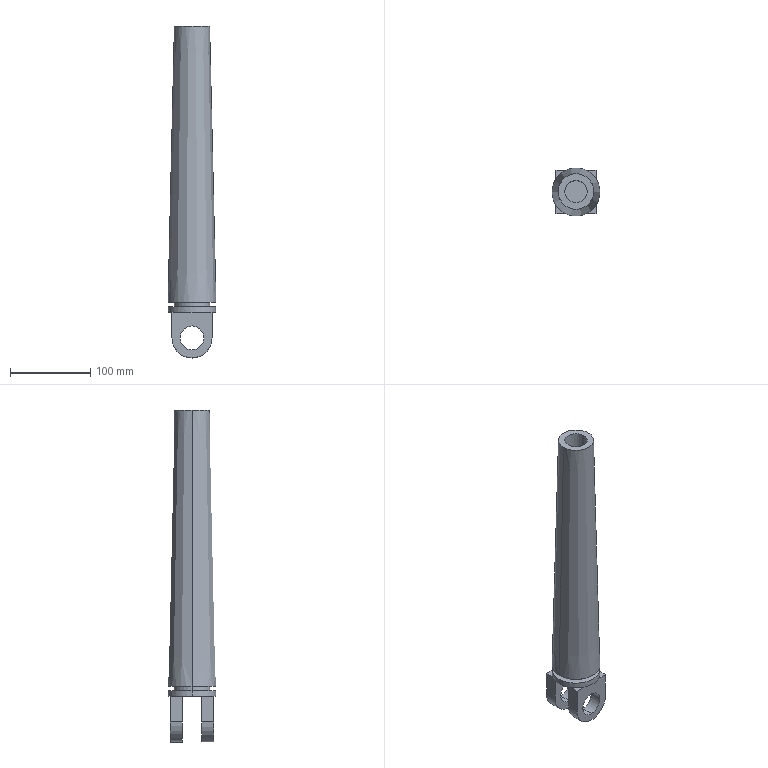Part | SolidWorks | features Extrusion 1, MirrorPattern 1, Revolution 1 | 1 solid | 34 faces | box 59.866 x 59.866 x 414.086 mm | volume 604728 mm3 | plane 19 | cylinder 13 | cone 2 | commonest cylinder face diameters 30 x4 50 x3 28 x2 44.765 x2 59.866 x2
STEP:
#1=CARTESIAN_POINT('',(0.,-39.,-15.));
#2=VERTEX_POINT('',#1);
#3=CARTESIAN_POINT('',(0.,-39.,15.));
#4=VERTEX_POINT('',#3);
#5=CARTESIAN_POINT('',(0.,-39.,0.));
#6=DIRECTION('',(0.,1.,0.));
#7=DIRECTION('',(0.,0.,1.));
#8=AXIS2_PLACEMENT_3D('',#5,#6,#7);
#9=CIRCLE('',#8,15.);
#10=EDGE_CURVE('',#2,#4,#9,.T.);
#11=ORIENTED_EDGE('',*,*,#10,.F.);
#12=CARTESIAN_POINT('',(0.,-24.,-15.));
#13=VERTEX_POINT('',#12);
#14=CARTESIAN_POINT('',(0.,-39.,-15.));
#15=DIRECTION('',(0.,1.,0.));
#16=VECTOR('',#15,1000.);
#17=LINE('',#14,#16);
#18=EDGE_CURVE('',#2,#13,#17,.T.);
#19=ORIENTED_EDGE('',*,*,#18,.T.);
#20=CARTESIAN_POINT('',(0.,-24.,15.));
#21=VERTEX_POINT('',#20);
#22=CARTESIAN_POINT('',(0.,-24.,0.));
#23=DIRECTION('',(0.,1.,0.));
#24=DIRECTION('',(0.,0.,1.));
#25=AXIS2_PLACEMENT_3D('',#22,#23,#24);
#26=CIRCLE('',#25,15.);
#27=EDGE_CURVE('',#13,#21,#26,.T.);
#28=ORIENTED_EDGE('',*,*,#27,.T.);
#29=CARTESIAN_POINT('',(0.,-39.,15.));
#30=DIRECTION('',(0.,1.,0.));
#31=VECTOR('',#30,1000.);
#32=LINE('',#29,#31);
#33=EDGE_CURVE('',#4,#21,#32,.T.);
#34=ORIENTED_EDGE('',*,*,#33,.F.);
#35=EDGE_LOOP('',(#11,#19,#28,#34));
#36=FACE_OUTER_BOUND('',#35,.T.);
#37=CARTESIAN_POINT('',(0.,-39.,0.));
#38=DIRECTION('',(0.,1.,0.));
#39=DIRECTION('',(0.,0.,1.));
#40=AXIS2_PLACEMENT_3D('',#37,#38,#39);
#41=CYLINDRICAL_SURFACE('',#40,15.);
#42=ADVANCED_FACE('',(#36),#41,.F.);
#43=CARTESIAN_POINT('',(-29.933,-12.,39.086));
#44=VERTEX_POINT('',#43);
#45=CARTESIAN_POINT('',(29.933,-12.,39.086));
#46=VERTEX_POINT('',#45);
#47=CARTESIAN_POINT('',(0.,-12.,39.086));
#48=DIRECTION('',(0.,0.,-1.));
#49=DIRECTION('',(-1.,0.,0.));
#50=AXIS2_PLACEMENT_3D('',#47,#48,#49);
#51=CIRCLE('',#50,29.933);
#52=EDGE_CURVE('',#44,#46,#51,.T.);
#53=ORIENTED_EDGE('',*,*,#52,.T.);
#54=CARTESIAN_POINT('',(29.933,-12.,31.913));
#55=VERTEX_POINT('',#54);
#56=CARTESIAN_POINT('',(29.933,-12.,31.913));
#57=DIRECTION('',(0.,0.,-1.));
#58=VECTOR('',#57,1000.);
#59=LINE('',#56,#58);
#60=EDGE_CURVE('',#46,#55,#59,.T.);
#61=ORIENTED_EDGE('',*,*,#60,.T.);
#62=CARTESIAN_POINT('',(25.,4.462,31.913));
#63=VERTEX_POINT('',#62);
#64=CARTESIAN_POINT('',(0.,-12.,31.913));
#65=DIRECTION('',(0.,0.,-1.));
#66=DIRECTION('',(-1.,0.,0.));
#67=AXIS2_PLACEMENT_3D('',#64,#65,#66);
#68=CIRCLE('',#67,29.933);
#69=EDGE_CURVE('',#63,#55,#68,.T.);
#70=ORIENTED_EDGE('',*,*,#69,.F.);
#71=CARTESIAN_POINT('',(12.923,15.,31.913));
#72=VERTEX_POINT('',#71);
#73=CARTESIAN_POINT('',(0.,-12.,31.913));
#74=DIRECTION('',(0.,0.,-1.));
#75=DIRECTION('',(-1.,0.,0.));
#76=AXIS2_PLACEMENT_3D('',#73,#74,#75);
#77=CIRCLE('',#76,29.933);
#78=EDGE_CURVE('',#72,#63,#77,.T.);
#79=ORIENTED_EDGE('',*,*,#78,.F.);
#80=CARTESIAN_POINT('',(-12.923,15.,31.913));
#81=VERTEX_POINT('',#80);
#82=CARTESIAN_POINT('',(0.,-12.,31.913));
#83=DIRECTION('',(0.,0.,-1.));
#84=DIRECTION('',(-1.,0.,0.));
#85=AXIS2_PLACEMENT_3D('',#82,#83,#84);
#86=CIRCLE('',#85,29.933);
#87=EDGE_CURVE('',#81,#72,#86,.T.);
#88=ORIENTED_EDGE('',*,*,#87,.F.);
#89=CARTESIAN_POINT('',(-25.,4.462,31.913));
#90=VERTEX_POINT('',#89);
#91=CARTESIAN_POINT('',(0.,-12.,31.913));
#92=DIRECTION('',(0.,0.,-1.));
#93=DIRECTION('',(-1.,0.,0.));
#94=AXIS2_PLACEMENT_3D('',#91,#92,#93);
#95=CIRCLE('',#94,29.933);
#96=EDGE_CURVE('',#90,#81,#95,.T.);
#97=ORIENTED_EDGE('',*,*,#96,.F.);
#98=CARTESIAN_POINT('',(-29.933,-12.,31.913));
#99=VERTEX_POINT('',#98);
#100=CARTESIAN_POINT('',(0.,-12.,31.913));
#101=DIRECTION('',(0.,0.,-1.));
#102=DIRECTION('',(-1.,0.,0.));
#103=AXIS2_PLACEMENT_3D('',#100,#101,#102);
#104=CIRCLE('',#103,29.933);
#105=EDGE_CURVE('',#99,#90,#104,.T.);
#106=ORIENTED_EDGE('',*,*,#105,.F.);
#107=CARTESIAN_POINT('',(-29.933,-12.,31.913));
#108=DIRECTION('',(0.,0.,-1.));
#109=VECTOR('',#108,1000.);
#110=LINE('',#107,#109);
#111=EDGE_CURVE('',#44,#99,#110,.T.);
#112=ORIENTED_EDGE('',*,*,#111,.F.);
#113=EDGE_LOOP('',(#53,#61,#70,#79,#88,#97,#106,#112));
#114=FACE_OUTER_BOUND('',#113,.T.);
#115=CARTESIAN_POINT('',(0.,-12.,31.913));
#116=DIRECTION('',(0.,0.,-1.));
#117=DIRECTION('',(-1.,0.,0.));
#118=AXIS2_PLACEMENT_3D('',#115,#116,#117);
#119=CYLINDRICAL_SURFACE('',#118,29.933);
#120=ADVANCED_FACE('',(#114),#119,.T.);
#121=CARTESIAN_POINT('',(-22.383,-12.,44.842));
#122=VERTEX_POINT('',#121);
#123=CARTESIAN_POINT('',(22.383,-12.,44.842));
#124=VERTEX_POINT('',#123);
#125=CARTESIAN_POINT('',(0.,-12.,44.842));
#126=DIRECTION('',(0.,0.,-1.));
#127=DIRECTION('',(-1.,0.,0.));
#128=AXIS2_PLACEMENT_3D('',#125,#126,#127);
#129=CIRCLE('',#128,22.383);
#130=EDGE_CURVE('',#122,#124,#129,.T.);
#131=ORIENTED_EDGE('',*,*,#130,.T.);
#132=CARTESIAN_POINT('',(22.383,-12.,39.086));
#133=VERTEX_POINT('',#132);
#134=CARTESIAN_POINT('',(22.383,-12.,31.913));
#135=DIRECTION('',(0.,0.,-1.));
#136=VECTOR('',#135,1000.);
#137=LINE('',#134,#136);
#138=EDGE_CURVE('',#124,#133,#137,.T.);
#139=ORIENTED_EDGE('',*,*,#138,.T.);
#140=CARTESIAN_POINT('',(-22.383,-12.,39.086));
#141=VERTEX_POINT('',#140);
#142=CARTESIAN_POINT('',(0.,-12.,39.086));
#143=DIRECTION('',(0.,0.,-1.));
#144=DIRECTION('',(-1.,0.,0.));
#145=AXIS2_PLACEMENT_3D('',#142,#143,#144);
#146=CIRCLE('',#145,22.383);
#147=EDGE_CURVE('',#141,#133,#146,.T.);
#148=ORIENTED_EDGE('',*,*,#147,.F.);
#149=CARTESIAN_POINT('',(-22.383,-12.,31.913));
#150=DIRECTION('',(0.,0.,-1.));
#151=VECTOR('',#150,1000.);
#152=LINE('',#149,#151);
#153=EDGE_CURVE('',#122,#141,#152,.T.);
#154=ORIENTED_EDGE('',*,*,#153,.F.);
#155=EDGE_LOOP('',(#131,#139,#148,#154));
#156=FACE_OUTER_BOUND('',#155,.T.);
#157=CARTESIAN_POINT('',(0.,-12.,31.913));
#158=DIRECTION('',(0.,0.,-1.));
#159=DIRECTION('',(-1.,0.,0.));
#160=AXIS2_PLACEMENT_3D('',#157,#158,#159);
#161=CYLINDRICAL_SURFACE('',#160,22.383);
#162=ADVANCED_FACE('',(#156),#161,.T.);
#163=CARTESIAN_POINT('',(-22.,-12.,389.086));
#164=VERTEX_POINT('',#163);
#165=CARTESIAN_POINT('',(22.,-12.,389.086));
#166=VERTEX_POINT('',#165);
#167=CARTESIAN_POINT('',(0.,-12.,389.086));
#168=DIRECTION('',(0.,0.,-1.));
#169=DIRECTION('',(-1.,0.,0.));
#170=AXIS2_PLACEMENT_3D('',#167,#168,#169);
#171=CIRCLE('',#170,22.);
#172=EDGE_CURVE('',#164,#166,#171,.T.);
#173=ORIENTED_EDGE('',*,*,#172,.T.);
#174=CARTESIAN_POINT('',(29.933,-12.,44.842));
#175=VERTEX_POINT('',#174);
#176=CARTESIAN_POINT('',(22.,-12.,389.086));
#177=DIRECTION('',(0.02304,0.,-0.9997));
#178=VECTOR('',#177,1000.);
#179=LINE('',#176,#178);
#180=EDGE_CURVE('',#166,#175,#179,.T.);
#181=ORIENTED_EDGE('',*,*,#180,.T.);
#182=CARTESIAN_POINT('',(-29.933,-12.,44.842));
#183=VERTEX_POINT('',#182);
#184=CARTESIAN_POINT('',(0.,-12.,44.842));
#185=DIRECTION('',(0.,0.,-1.));
#186=DIRECTION('',(-1.,0.,0.));
#187=AXIS2_PLACEMENT_3D('',#184,#185,#186);
#188=CIRCLE('',#187,29.933);
#189=EDGE_CURVE('',#183,#175,#188,.T.);
#190=ORIENTED_EDGE('',*,*,#189,.F.);
#191=CARTESIAN_POINT('',(-22.,-12.,389.086));
#192=DIRECTION('',(-0.02304,0.,-0.9997));
#193=VECTOR('',#192,1000.);
#194=LINE('',#191,#193);
#195=EDGE_CURVE('',#164,#183,#194,.T.);
#196=ORIENTED_EDGE('',*,*,#195,.F.);
#197=EDGE_LOOP('',(#173,#181,#190,#196));
#198=FACE_OUTER_BOUND('',#197,.T.);
#199=CARTESIAN_POINT('',(0.,-12.,389.086));
#200=DIRECTION('',(0.,0.,-1.));
#201=DIRECTION('',(-1.,0.,0.));
#202=AXIS2_PLACEMENT_3D('',#199,#200,#201);
#203=CONICAL_SURFACE('',#202,22.,0.02304);
#204=ADVANCED_FACE('',(#198),#203,.T.);
#205=CARTESIAN_POINT('',(14.,-12.,389.086));
#206=VERTEX_POINT('',#205);
#207=CARTESIAN_POINT('',(-14.,-12.,389.086));
#208=VERTEX_POINT('',#207);
#209=CARTESIAN_POINT('',(0.,-12.,389.086));
#210=DIRECTION('',(0.,0.,-1.));
#211=DIRECTION('',(-1.,0.,0.));
#212=AXIS2_PLACEMENT_3D('',#209,#210,#211);
#213=CIRCLE('',#212,14.);
#214=EDGE_CURVE('',#206,#208,#213,.T.);
#215=ORIENTED_EDGE('',*,*,#214,.F.);
#216=CARTESIAN_POINT('',(14.,-12.,39.086));
#217=VERTEX_POINT('',#216);
#218=CARTESIAN_POINT('',(14.,-12.,31.913));
#219=DIRECTION('',(0.,0.,-1.));
#220=VECTOR('',#219,1000.);
#221=LINE('',#218,#220);
#222=EDGE_CURVE('',#206,#217,#221,.T.);
#223=ORIENTED_EDGE('',*,*,#222,.T.);
#224=CARTESIAN_POINT('',(-14.,-12.,39.086));
#225=VERTEX_POINT('',#224);
#226=CARTESIAN_POINT('',(0.,-12.,39.086));
#227=DIRECTION('',(0.,0.,-1.));
#228=DIRECTION('',(-1.,0.,0.));
#229=AXIS2_PLACEMENT_3D('',#226,#227,#228);
#230=CIRCLE('',#229,14.);
#231=EDGE_CURVE('',#217,#225,#230,.T.);
#232=ORIENTED_EDGE('',*,*,#231,.T.);
#233=CARTESIAN_POINT('',(-14.,-12.,31.913));
#234=DIRECTION('',(0.,0.,-1.));
#235=VECTOR('',#234,1000.);
#236=LINE('',#233,#235);
#237=EDGE_CURVE('',#208,#225,#236,.T.);
#238=ORIENTED_EDGE('',*,*,#237,.F.);
#239=EDGE_LOOP('',(#215,#223,#232,#238));
#240=FACE_OUTER_BOUND('',#239,.T.);
#241=CARTESIAN_POINT('',(0.,-12.,31.913));
#242=DIRECTION('',(0.,0.,-1.));
#243=DIRECTION('',(-1.,0.,0.));
#244=AXIS2_PLACEMENT_3D('',#241,#242,#243);
#245=CYLINDRICAL_SURFACE('',#244,14.);
#246=ADVANCED_FACE('',(#240),#245,.F.);
#247=CARTESIAN_POINT('',(0.,15.,-15.));
#248=VERTEX_POINT('',#247);
#249=CARTESIAN_POINT('',(0.,15.,15.));
#250=VERTEX_POINT('',#249);
#251=CARTESIAN_POINT('',(0.,15.,0.));
#252=DIRECTION('',(0.,1.,0.));
#253=DIRECTION('',(0.,0.,1.));
#254=AXIS2_PLACEMENT_3D('',#251,#252,#253);
#255=CIRCLE('',#254,15.);
#256=EDGE_CURVE('',#248,#250,#255,.T.);
#257=ORIENTED_EDGE('',*,*,#256,.T.);
#258=CARTESIAN_POINT('',(0.,0.,15.));
#259=VERTEX_POINT('',#258);
#260=CARTESIAN_POINT('',(0.,15.,15.));
#261=DIRECTION('',(0.,-1.,0.));
#262=VECTOR('',#261,1000.);
#263=LINE('',#260,#262);
#264=EDGE_CURVE('',#250,#259,#263,.T.);
#265=ORIENTED_EDGE('',*,*,#264,.T.);
#266=CARTESIAN_POINT('',(0.,0.,-15.));
#267=VERTEX_POINT('',#266);
#268=CARTESIAN_POINT('',(0.,0.,0.));
#269=DIRECTION('',(0.,1.,0.));
#270=DIRECTION('',(0.,0.,1.));
#271=AXIS2_PLACEMENT_3D('',#268,#269,#270);
#272=CIRCLE('',#271,15.);
#273=EDGE_CURVE('',#267,#259,#272,.T.);
#274=ORIENTED_EDGE('',*,*,#273,.F.);
#275=CARTESIAN_POINT('',(0.,15.,-15.));
#276=DIRECTION('',(0.,-1.,0.));
#277=VECTOR('',#276,1000.);
#278=LINE('',#275,#277);
#279=EDGE_CURVE('',#248,#267,#278,.T.);
#280=ORIENTED_EDGE('',*,*,#279,.F.);
#281=EDGE_LOOP('',(#257,#265,#274,#280));
#282=FACE_OUTER_BOUND('',#281,.T.);
#283=CARTESIAN_POINT('',(0.,15.,0.));
#284=DIRECTION('',(0.,-1.,0.));
#285=DIRECTION('',(0.,0.,-1.));
#286=AXIS2_PLACEMENT_3D('',#283,#284,#285);
#287=CYLINDRICAL_SURFACE('',#286,15.);
#288=ADVANCED_FACE('',(#282),#287,.F.);
#289=CARTESIAN_POINT('',(0.,15.,-25.));
#290=VERTEX_POINT('',#289);
#291=CARTESIAN_POINT('',(-25.,15.,0.));
#292=VERTEX_POINT('',#291);
#293=CARTESIAN_POINT('',(0.,15.,0.));
#294=DIRECTION('',(0.,1.,0.));
#295=DIRECTION('',(0.,0.,1.));
#296=AXIS2_PLACEMENT_3D('',#293,#294,#295);
#297=CIRCLE('',#296,25.);
#298=EDGE_CURVE('',#290,#292,#297,.T.);
#299=ORIENTED_EDGE('',*,*,#298,.F.);
#300=CARTESIAN_POINT('',(0.,0.,-25.));
#301=VERTEX_POINT('',#300);
#302=CARTESIAN_POINT('',(0.,15.,-25.));
#303=DIRECTION('',(0.,-1.,0.));
#304=VECTOR('',#303,1000.);
#305=LINE('',#302,#304);
#306=EDGE_CURVE('',#290,#301,#305,.T.);
#307=ORIENTED_EDGE('',*,*,#306,.T.);
#308=CARTESIAN_POINT('',(-25.,0.,0.));
#309=VERTEX_POINT('',#308);
#310=CARTESIAN_POINT('',(0.,0.,0.));
#311=DIRECTION('',(0.,1.,0.));
#312=DIRECTION('',(0.,0.,1.));
#313=AXIS2_PLACEMENT_3D('',#310,#311,#312);
#314=CIRCLE('',#313,25.);
#315=EDGE_CURVE('',#301,#309,#314,.T.);
#316=ORIENTED_EDGE('',*,*,#315,.T.);
#317=CARTESIAN_POINT('',(-25.,15.,0.));
#318=DIRECTION('',(0.,-1.,0.));
#319=VECTOR('',#318,1000.);
#320=LINE('',#317,#319);
#321=EDGE_CURVE('',#292,#309,#320,.T.);
#322=ORIENTED_EDGE('',*,*,#321,.F.);
#323=EDGE_LOOP('',(#299,#307,#316,#322));
#324=FACE_OUTER_BOUND('',#323,.T.);
#325=CARTESIAN_POINT('',(0.,15.,0.));
#326=DIRECTION('',(0.,-1.,0.));
#327=DIRECTION('',(0.,0.,-1.));
#328=AXIS2_PLACEMENT_3D('',#325,#326,#327);
#329=CYLINDRICAL_SURFACE('',#328,25.);
#330=ADVANCED_FACE('',(#324),#329,.T.);
#331=CARTESIAN_POINT('',(12.923,-39.,31.913));
#332=VERTEX_POINT('',#331);
#333=CARTESIAN_POINT('',(-12.923,-39.,31.913));
#334=VERTEX_POINT('',#333);
#335=CARTESIAN_POINT('',(0.,-12.,31.913));
#336=DIRECTION('',(0.,0.,-1.));
#337=DIRECTION('',(-1.,0.,0.));
#338=AXIS2_PLACEMENT_3D('',#335,#336,#337);
#339=CIRCLE('',#338,29.933);
#340=EDGE_CURVE('',#332,#334,#339,.T.);
#341=ORIENTED_EDGE('',*,*,#340,.T.);
#342=CARTESIAN_POINT('',(0.,-39.,31.913));
#343=DIRECTION('',(1.,0.,0.));
#344=VECTOR('',#343,1000.);
#345=LINE('',#342,#344);
#346=EDGE_CURVE('',#334,#332,#345,.T.);
#347=ORIENTED_EDGE('',*,*,#346,.T.);
#348=EDGE_LOOP('',(#341,#347));
#349=FACE_OUTER_BOUND('',#348,.T.);
#350=CARTESIAN_POINT('',(0.,-12.,31.913));
#351=DIRECTION('',(0.,0.,1.));
#352=DIRECTION('',(1.,0.,0.));
#353=AXIS2_PLACEMENT_3D('',#350,#351,#352);
#354=PLANE('',#353);
#355=ADVANCED_FACE('',(#349),#354,.F.);
#356=CARTESIAN_POINT('',(-25.,15.,31.913));
#357=VERTEX_POINT('',#356);
#358=CARTESIAN_POINT('',(-25.,15.,31.913));
#359=DIRECTION('',(0.,-1.,0.));
#360=VECTOR('',#359,1000.);
#361=LINE('',#358,#360);
#362=EDGE_CURVE('',#357,#90,#361,.T.);
#363=ORIENTED_EDGE('',*,*,#362,.T.);
#364=ORIENTED_EDGE('',*,*,#96,.T.);
#365=CARTESIAN_POINT('',(-25.,15.,31.913));
#366=DIRECTION('',(1.,0.,0.));
#367=VECTOR('',#366,1000.);
#368=LINE('',#365,#367);
#369=EDGE_CURVE('',#357,#81,#368,.T.);
#370=ORIENTED_EDGE('',*,*,#369,.F.);
#371=EDGE_LOOP('',(#363,#364,#370));
#372=FACE_OUTER_BOUND('',#371,.T.);
#373=CARTESIAN_POINT('',(-25.,15.,31.913));
#374=DIRECTION('',(0.,0.,-1.));
#375=DIRECTION('',(-1.,0.,0.));
#376=AXIS2_PLACEMENT_3D('',#373,#374,#375);
#377=PLANE('',#376);
#378=ADVANCED_FACE('',(#372),#377,.F.);
#379=CARTESIAN_POINT('',(25.,15.,0.));
#380=VERTEX_POINT('',#379);
#381=CARTESIAN_POINT('',(0.,15.,0.));
#382=DIRECTION('',(0.,1.,0.));
#383=DIRECTION('',(0.,0.,1.));
#384=AXIS2_PLACEMENT_3D('',#381,#382,#383);
#385=CIRCLE('',#384,25.);
#386=EDGE_CURVE('',#380,#290,#385,.T.);
#387=ORIENTED_EDGE('',*,*,#386,.T.);
#388=ORIENTED_EDGE('',*,*,#298,.T.);
#389=CARTESIAN_POINT('',(-25.,15.,0.));
#390=DIRECTION('',(0.,0.,1.));
#391=VECTOR('',#390,1000.);
#392=LINE('',#389,#391);
#393=EDGE_CURVE('',#292,#357,#392,.T.);
#394=ORIENTED_EDGE('',*,*,#393,.T.);
#395=ORIENTED_EDGE('',*,*,#369,.T.);
#396=CARTESIAN_POINT('',(-25.,15.,31.913));
#397=DIRECTION('',(1.,0.,0.));
#398=VECTOR('',#397,1000.);
#399=LINE('',#396,#398);
#400=EDGE_CURVE('',#81,#72,#399,.T.);
#401=ORIENTED_EDGE('',*,*,#400,.T.);
#402=CARTESIAN_POINT('',(25.,15.,31.913));
#403=VERTEX_POINT('',#402);
#404=CARTESIAN_POINT('',(-25.,15.,31.913));
#405=DIRECTION('',(1.,0.,0.));
#406=VECTOR('',#405,1000.);
#407=LINE('',#404,#406);
#408=EDGE_CURVE('',#72,#403,#407,.T.);
#409=ORIENTED_EDGE('',*,*,#408,.T.);
#410=CARTESIAN_POINT('',(25.,15.,0.));
#411=DIRECTION('',(0.,0.,-1.));
#412=VECTOR('',#411,1000.);
#413=LINE('',#410,#412);
#414=EDGE_CURVE('',#403,#380,#413,.T.);
#415=ORIENTED_EDGE('',*,*,#414,.T.);
#416=EDGE_LOOP('',(#387,#388,#394,#395,#401,#409,#415));
#417=FACE_OUTER_BOUND('',#416,.T.);
#418=ORIENTED_EDGE('',*,*,#256,.F.);
#419=CARTESIAN_POINT('',(0.,15.,0.));
#420=DIRECTION('',(0.,1.,0.));
#421=DIRECTION('',(0.,0.,1.));
#422=AXIS2_PLACEMENT_3D('',#419,#420,#421);
#423=CIRCLE('',#422,15.);
#424=EDGE_CURVE('',#250,#248,#423,.T.);
#425=ORIENTED_EDGE('',*,*,#424,.F.);
#426=EDGE_LOOP('',(#418,#425));
#427=FACE_BOUND('',#426,.T.);
#428=CARTESIAN_POINT('',(0.,15.,0.));
#429=DIRECTION('',(0.,1.,0.));
#430=DIRECTION('',(0.,0.,1.));
#431=AXIS2_PLACEMENT_3D('',#428,#429,#430);
#432=PLANE('',#431);
#433=ADVANCED_FACE('',(#417,#427),#432,.T.);
#434=CARTESIAN_POINT('',(25.,0.,0.));
#435=VERTEX_POINT('',#434);
#436=CARTESIAN_POINT('',(0.,0.,0.));
#437=DIRECTION('',(0.,1.,0.));
#438=DIRECTION('',(0.,0.,1.));
#439=AXIS2_PLACEMENT_3D('',#436,#437,#438);
#440=CIRCLE('',#439,25.);
#441=EDGE_CURVE('',#435,#301,#440,.T.);
#442=ORIENTED_EDGE('',*,*,#441,.F.);
#443=CARTESIAN_POINT('',(25.,0.,31.913));
#444=VERTEX_POINT('',#443);
#445=CARTESIAN_POINT('',(25.,0.,0.));
#446=DIRECTION('',(0.,0.,-1.));
#447=VECTOR('',#446,1000.);
#448=LINE('',#445,#447);
#449=EDGE_CURVE('',#444,#435,#448,.T.);
#450=ORIENTED_EDGE('',*,*,#449,.F.);
#451=CARTESIAN_POINT('',(-25.,0.,31.913));
#452=VERTEX_POINT('',#451);
#453=CARTESIAN_POINT('',(-25.,0.,31.913));
#454=DIRECTION('',(1.,0.,0.));
#455=VECTOR('',#454,1000.);
#456=LINE('',#453,#455);
#457=EDGE_CURVE('',#452,#444,#456,.T.);
#458=ORIENTED_EDGE('',*,*,#457,.F.);
#459=CARTESIAN_POINT('',(-25.,0.,0.));
#460=DIRECTION('',(0.,0.,1.));
#461=VECTOR('',#460,1000.);
#462=LINE('',#459,#461);
#463=EDGE_CURVE('',#309,#452,#462,.T.);
#464=ORIENTED_EDGE('',*,*,#463,.F.);
#465=ORIENTED_EDGE('',*,*,#315,.F.);
#466=EDGE_LOOP('',(#442,#450,#458,#464,#465));
#467=FACE_OUTER_BOUND('',#466,.T.);
#468=ORIENTED_EDGE('',*,*,#273,.T.);
#469=CARTESIAN_POINT('',(0.,0.,0.));
#470=DIRECTION('',(0.,1.,0.));
#471=DIRECTION('',(0.,0.,1.));
#472=AXIS2_PLACEMENT_3D('',#469,#470,#471);
#473=CIRCLE('',#472,15.);
#474=EDGE_CURVE('',#259,#267,#473,.T.);
#475=ORIENTED_EDGE('',*,*,#474,.T.);
#476=EDGE_LOOP('',(#468,#475));
#477=FACE_BOUND('',#476,.T.);
#478=CARTESIAN_POINT('',(0.,0.,0.));
#479=DIRECTION('',(0.,1.,0.));
#480=DIRECTION('',(0.,0.,1.));
#481=AXIS2_PLACEMENT_3D('',#478,#479,#480);
#482=PLANE('',#481);
#483=ADVANCED_FACE('',(#467,#477),#482,.F.);
#484=ORIENTED_EDGE('',*,*,#306,.F.);
#485=ORIENTED_EDGE('',*,*,#386,.F.);
#486=CARTESIAN_POINT('',(25.,15.,0.));
#487=DIRECTION('',(0.,-1.,0.));
#488=VECTOR('',#487,1000.);
#489=LINE('',#486,#488);
#490=EDGE_CURVE('',#380,#435,#489,.T.);
#491=ORIENTED_EDGE('',*,*,#490,.T.);
#492=ORIENTED_EDGE('',*,*,#441,.T.);
#493=EDGE_LOOP('',(#484,#485,#491,#492));
#494=FACE_OUTER_BOUND('',#493,.T.);
#495=CARTESIAN_POINT('',(0.,15.,0.));
#496=DIRECTION('',(0.,-1.,0.));
#497=DIRECTION('',(0.,0.,-1.));
#498=AXIS2_PLACEMENT_3D('',#495,#496,#497);
#499=CYLINDRICAL_SURFACE('',#498,25.);
#500=ADVANCED_FACE('',(#494),#499,.T.);
#501=ORIENTED_EDGE('',*,*,#463,.T.);
#502=CARTESIAN_POINT('',(-25.,15.,31.913));
#503=DIRECTION('',(0.,-1.,0.));
#504=VECTOR('',#503,1000.);
#505=LINE('',#502,#504);
#506=EDGE_CURVE('',#90,#452,#505,.T.);
#507=ORIENTED_EDGE('',*,*,#506,.F.);
#508=ORIENTED_EDGE('',*,*,#362,.F.);
#509=ORIENTED_EDGE('',*,*,#393,.F.);
#510=ORIENTED_EDGE('',*,*,#321,.T.);
#511=EDGE_LOOP('',(#501,#507,#508,#509,#510));
#512=FACE_OUTER_BOUND('',#511,.T.);
#513=CARTESIAN_POINT('',(-25.,15.,0.));
#514=DIRECTION('',(1.,0.,0.));
#515=DIRECTION('',(0.,0.,-1.));
#516=AXIS2_PLACEMENT_3D('',#513,#514,#515);
#517=PLANE('',#516);
#518=ADVANCED_FACE('',(#512),#517,.F.);
#519=ORIENTED_EDGE('',*,*,#408,.F.);
#520=ORIENTED_EDGE('',*,*,#78,.T.);
#521=CARTESIAN_POINT('',(25.,15.,31.913));
#522=DIRECTION('',(0.,-1.,0.));
#523=VECTOR('',#522,1000.);
#524=LINE('',#521,#523);
#525=EDGE_CURVE('',#403,#63,#524,.T.);
#526=ORIENTED_EDGE('',*,*,#525,.F.);
#527=EDGE_LOOP('',(#519,#520,#526));
#528=FACE_OUTER_BOUND('',#527,.T.);
#529=CARTESIAN_POINT('',(-25.,15.,31.913));
#530=DIRECTION('',(0.,0.,-1.));
#531=DIRECTION('',(-1.,0.,0.));
#532=AXIS2_PLACEMENT_3D('',#529,#530,#531);
#533=PLANE('',#532);
#534=ADVANCED_FACE('',(#528),#533,.F.);
#535=ORIENTED_EDGE('',*,*,#449,.T.);
#536=ORIENTED_EDGE('',*,*,#490,.F.);
#537=ORIENTED_EDGE('',*,*,#414,.F.);
#538=ORIENTED_EDGE('',*,*,#525,.T.);
#539=CARTESIAN_POINT('',(25.,15.,31.913));
#540=DIRECTION('',(0.,-1.,0.));
#541=VECTOR('',#540,1000.);
#542=LINE('',#539,#541);
#543=EDGE_CURVE('',#63,#444,#542,.T.);
#544=ORIENTED_EDGE('',*,*,#543,.T.);
#545=EDGE_LOOP('',(#535,#536,#537,#538,#544));
#546=FACE_OUTER_BOUND('',#545,.T.);
#547=CARTESIAN_POINT('',(25.,15.,0.));
#548=DIRECTION('',(-1.,0.,0.));
#549=DIRECTION('',(0.,0.,1.));
#550=AXIS2_PLACEMENT_3D('',#547,#548,#549);
#551=PLANE('',#550);
#552=ADVANCED_FACE('',(#546),#551,.F.);
#553=ORIENTED_EDGE('',*,*,#264,.F.);
#554=ORIENTED_EDGE('',*,*,#424,.T.);
#555=ORIENTED_EDGE('',*,*,#279,.T.);
#556=ORIENTED_EDGE('',*,*,#474,.F.);
#557=EDGE_LOOP('',(#553,#554,#555,#556));
#558=FACE_OUTER_BOUND('',#557,.T.);
#559=CARTESIAN_POINT('',(0.,15.,0.));
#560=DIRECTION('',(0.,-1.,0.));
#561=DIRECTION('',(0.,0.,-1.));
#562=AXIS2_PLACEMENT_3D('',#559,#560,#561);
#563=CYLINDRICAL_SURFACE('',#562,15.);
#564=ADVANCED_FACE('',(#558),#563,.F.);
#565=ORIENTED_EDGE('',*,*,#400,.F.);
#566=ORIENTED_EDGE('',*,*,#87,.T.);
#567=EDGE_LOOP('',(#565,#566));
#568=FACE_OUTER_BOUND('',#567,.T.);
#569=CARTESIAN_POINT('',(0.,-12.,31.913));
#570=DIRECTION('',(0.,0.,1.));
#571=DIRECTION('',(1.,0.,0.));
#572=AXIS2_PLACEMENT_3D('',#569,#570,#571);
#573=PLANE('',#572);
#574=ADVANCED_FACE('',(#568),#573,.F.);
#575=CARTESIAN_POINT('',(0.,-12.,39.086));
#576=DIRECTION('',(0.,0.,-1.));
#577=DIRECTION('',(-1.,0.,0.));
#578=AXIS2_PLACEMENT_3D('',#575,#576,#577);
#579=CIRCLE('',#578,14.);
#580=EDGE_CURVE('',#225,#217,#579,.T.);
#581=ORIENTED_EDGE('',*,*,#580,.F.);
#582=ORIENTED_EDGE('',*,*,#231,.F.);
#583=EDGE_LOOP('',(#581,#582));
#584=FACE_OUTER_BOUND('',#583,.T.);
#585=CARTESIAN_POINT('',(0.,-12.,39.086));
#586=DIRECTION('',(0.,0.,-1.));
#587=DIRECTION('',(-1.,0.,0.));
#588=AXIS2_PLACEMENT_3D('',#585,#586,#587);
#589=PLANE('',#588);
#590=ADVANCED_FACE('',(#584),#589,.F.);
#591=ORIENTED_EDGE('',*,*,#222,.F.);
#592=CARTESIAN_POINT('',(0.,-12.,389.086));
#593=DIRECTION('',(0.,0.,-1.));
#594=DIRECTION('',(-1.,0.,0.));
#595=AXIS2_PLACEMENT_3D('',#592,#593,#594);
#596=CIRCLE('',#595,14.);
#597=EDGE_CURVE('',#208,#206,#596,.T.);
#598=ORIENTED_EDGE('',*,*,#597,.F.);
#599=ORIENTED_EDGE('',*,*,#237,.T.);
#600=ORIENTED_EDGE('',*,*,#580,.T.);
#601=EDGE_LOOP('',(#591,#598,#599,#600));
#602=FACE_OUTER_BOUND('',#601,.T.);
#603=CARTESIAN_POINT('',(0.,-12.,31.913));
#604=DIRECTION('',(0.,0.,-1.));
#605=DIRECTION('',(-1.,0.,0.));
#606=AXIS2_PLACEMENT_3D('',#603,#604,#605);
#607=CYLINDRICAL_SURFACE('',#606,14.);
#608=ADVANCED_FACE('',(#602),#607,.F.);
#609=ORIENTED_EDGE('',*,*,#172,.F.);
#610=CARTESIAN_POINT('',(0.,-12.,389.086));
#611=DIRECTION('',(0.,0.,-1.));
#612=DIRECTION('',(-1.,0.,0.));
#613=AXIS2_PLACEMENT_3D('',#610,#611,#612);
#614=CIRCLE('',#613,22.);
#615=EDGE_CURVE('',#166,#164,#614,.T.);
#616=ORIENTED_EDGE('',*,*,#615,.F.);
#617=EDGE_LOOP('',(#609,#616));
#618=FACE_OUTER_BOUND('',#617,.T.);
#619=ORIENTED_EDGE('',*,*,#597,.T.);
#620=ORIENTED_EDGE('',*,*,#214,.T.);
#621=EDGE_LOOP('',(#619,#620));
#622=FACE_BOUND('',#621,.T.);
#623=CARTESIAN_POINT('',(-14.,-12.,389.086));
#624=DIRECTION('',(0.,0.,-1.));
#625=DIRECTION('',(-1.,0.,0.));
#626=AXIS2_PLACEMENT_3D('',#623,#624,#625);
#627=PLANE('',#626);
#628=ADVANCED_FACE('',(#618,#622),#627,.F.);
#629=ORIENTED_EDGE('',*,*,#180,.F.);
#630=ORIENTED_EDGE('',*,*,#615,.T.);
#631=ORIENTED_EDGE('',*,*,#195,.T.);
#632=CARTESIAN_POINT('',(0.,-12.,44.842));
#633=DIRECTION('',(0.,0.,-1.));
#634=DIRECTION('',(-1.,0.,0.));
#635=AXIS2_PLACEMENT_3D('',#632,#633,#634);
#636=CIRCLE('',#635,29.933);
#637=EDGE_CURVE('',#175,#183,#636,.T.);
#638=ORIENTED_EDGE('',*,*,#637,.F.);
#639=EDGE_LOOP('',(#629,#630,#631,#638));
#640=FACE_OUTER_BOUND('',#639,.T.);
#641=CARTESIAN_POINT('',(0.,-12.,389.086));
#642=DIRECTION('',(0.,0.,-1.));
#643=DIRECTION('',(-1.,0.,0.));
#644=AXIS2_PLACEMENT_3D('',#641,#642,#643);
#645=CONICAL_SURFACE('',#644,22.,0.02304);
#646=ADVANCED_FACE('',(#640),#645,.T.);
#647=ORIENTED_EDGE('',*,*,#130,.F.);
#648=CARTESIAN_POINT('',(0.,-12.,44.842));
#649=DIRECTION('',(0.,0.,-1.));
#650=DIRECTION('',(-1.,0.,0.));
#651=AXIS2_PLACEMENT_3D('',#648,#649,#650);
#652=CIRCLE('',#651,22.383);
#653=EDGE_CURVE('',#124,#122,#652,.T.);
#654=ORIENTED_EDGE('',*,*,#653,.F.);
#655=EDGE_LOOP('',(#647,#654));
#656=FACE_BOUND('',#655,.T.);
#657=ORIENTED_EDGE('',*,*,#189,.T.);
#658=ORIENTED_EDGE('',*,*,#637,.T.);
#659=EDGE_LOOP('',(#657,#658));
#660=FACE_OUTER_BOUND('',#659,.T.);
#661=CARTESIAN_POINT('',(-22.383,-12.,44.842));
#662=DIRECTION('',(0.,0.,1.));
#663=DIRECTION('',(1.,0.,0.));
#664=AXIS2_PLACEMENT_3D('',#661,#662,#663);
#665=PLANE('',#664);
#666=ADVANCED_FACE('',(#656,#660),#665,.F.);
#667=ORIENTED_EDGE('',*,*,#138,.F.);
#668=ORIENTED_EDGE('',*,*,#653,.T.);
#669=ORIENTED_EDGE('',*,*,#153,.T.);
#670=CARTESIAN_POINT('',(0.,-12.,39.086));
#671=DIRECTION('',(0.,0.,-1.));
#672=DIRECTION('',(-1.,0.,0.));
#673=AXIS2_PLACEMENT_3D('',#670,#671,#672);
#674=CIRCLE('',#673,22.383);
#675=EDGE_CURVE('',#133,#141,#674,.T.);
#676=ORIENTED_EDGE('',*,*,#675,.F.);
#677=EDGE_LOOP('',(#667,#668,#669,#676));
#678=FACE_OUTER_BOUND('',#677,.T.);
#679=CARTESIAN_POINT('',(0.,-12.,31.913));
#680=DIRECTION('',(0.,0.,-1.));
#681=DIRECTION('',(-1.,0.,0.));
#682=AXIS2_PLACEMENT_3D('',#679,#680,#681);
#683=CYLINDRICAL_SURFACE('',#682,22.383);
#684=ADVANCED_FACE('',(#678),#683,.T.);
#685=ORIENTED_EDGE('',*,*,#52,.F.);
#686=CARTESIAN_POINT('',(0.,-12.,39.086));
#687=DIRECTION('',(0.,0.,-1.));
#688=DIRECTION('',(-1.,0.,0.));
#689=AXIS2_PLACEMENT_3D('',#686,#687,#688);
#690=CIRCLE('',#689,29.933);
#691=EDGE_CURVE('',#46,#44,#690,.T.);
#692=ORIENTED_EDGE('',*,*,#691,.F.);
#693=EDGE_LOOP('',(#685,#692));
#694=FACE_OUTER_BOUND('',#693,.T.);
#695=ORIENTED_EDGE('',*,*,#147,.T.);
#696=ORIENTED_EDGE('',*,*,#675,.T.);
#697=EDGE_LOOP('',(#695,#696));
#698=FACE_BOUND('',#697,.T.);
#699=CARTESIAN_POINT('',(-29.933,-12.,39.086));
#700=DIRECTION('',(0.,0.,-1.));
#701=DIRECTION('',(-1.,0.,0.));
#702=AXIS2_PLACEMENT_3D('',#699,#700,#701);
#703=PLANE('',#702);
#704=ADVANCED_FACE('',(#694,#698),#703,.F.);
#705=ORIENTED_EDGE('',*,*,#60,.F.);
#706=ORIENTED_EDGE('',*,*,#691,.T.);
#707=ORIENTED_EDGE('',*,*,#111,.T.);
#708=CARTESIAN_POINT('',(-25.,-28.462,31.913));
#709=VERTEX_POINT('',#708);
#710=CARTESIAN_POINT('',(0.,-12.,31.913));
#711=DIRECTION('',(0.,0.,-1.));
#712=DIRECTION('',(-1.,0.,0.));
#713=AXIS2_PLACEMENT_3D('',#710,#711,#712);
#714=CIRCLE('',#713,29.933);
#715=EDGE_CURVE('',#709,#99,#714,.T.);
#716=ORIENTED_EDGE('',*,*,#715,.F.);
#717=CARTESIAN_POINT('',(0.,-12.,31.913));
#718=DIRECTION('',(0.,0.,-1.));
#719=DIRECTION('',(-1.,0.,0.));
#720=AXIS2_PLACEMENT_3D('',#717,#718,#719);
#721=CIRCLE('',#720,29.933);
#722=EDGE_CURVE('',#334,#709,#721,.T.);
#723=ORIENTED_EDGE('',*,*,#722,.F.);
#724=ORIENTED_EDGE('',*,*,#340,.F.);
#725=CARTESIAN_POINT('',(25.,-28.462,31.913));
#726=VERTEX_POINT('',#725);
#727=CARTESIAN_POINT('',(0.,-12.,31.913));
#728=DIRECTION('',(0.,0.,-1.));
#729=DIRECTION('',(-1.,0.,0.));
#730=AXIS2_PLACEMENT_3D('',#727,#728,#729);
#731=CIRCLE('',#730,29.933);
#732=EDGE_CURVE('',#726,#332,#731,.T.);
#733=ORIENTED_EDGE('',*,*,#732,.F.);
#734=CARTESIAN_POINT('',(0.,-12.,31.913));
#735=DIRECTION('',(0.,0.,-1.));
#736=DIRECTION('',(-1.,0.,0.));
#737=AXIS2_PLACEMENT_3D('',#734,#735,#736);
#738=CIRCLE('',#737,29.933);
#739=EDGE_CURVE('',#55,#726,#738,.T.);
#740=ORIENTED_EDGE('',*,*,#739,.F.);
#741=EDGE_LOOP('',(#705,#706,#707,#716,#723,#724,#733,#740));
#742=FACE_OUTER_BOUND('',#741,.T.);
#743=CARTESIAN_POINT('',(0.,-12.,31.913));
#744=DIRECTION('',(0.,0.,-1.));
#745=DIRECTION('',(-1.,0.,0.));
#746=AXIS2_PLACEMENT_3D('',#743,#744,#745);
#747=CYLINDRICAL_SURFACE('',#746,29.933);
#748=ADVANCED_FACE('',(#742),#747,.T.);
#749=ORIENTED_EDGE('',*,*,#69,.T.);
#750=ORIENTED_EDGE('',*,*,#739,.T.);
#751=CARTESIAN_POINT('',(25.,-24.,31.913));
#752=VERTEX_POINT('',#751);
#753=CARTESIAN_POINT('',(25.,-12.,31.913));
#754=DIRECTION('',(0.,1.,0.));
#755=VECTOR('',#754,1000.);
#756=LINE('',#753,#755);
#757=EDGE_CURVE('',#726,#752,#756,.T.);
#758=ORIENTED_EDGE('',*,*,#757,.T.);
#759=CARTESIAN_POINT('',(-25.,-24.,31.913));
#760=VERTEX_POINT('',#759);
#761=CARTESIAN_POINT('',(-25.,-24.,31.913));
#762=DIRECTION('',(1.,0.,0.));
#763=VECTOR('',#762,1000.);
#764=LINE('',#761,#763);
#765=EDGE_CURVE('',#760,#752,#764,.T.);
#766=ORIENTED_EDGE('',*,*,#765,.F.);
#767=CARTESIAN_POINT('',(-25.,-12.,31.913));
#768=DIRECTION('',(0.,-1.,0.));
#769=VECTOR('',#768,1000.);
#770=LINE('',#767,#769);
#771=EDGE_CURVE('',#760,#709,#770,.T.);
#772=ORIENTED_EDGE('',*,*,#771,.T.);
#773=ORIENTED_EDGE('',*,*,#715,.T.);
#774=ORIENTED_EDGE('',*,*,#105,.T.);
#775=ORIENTED_EDGE('',*,*,#506,.T.);
#776=ORIENTED_EDGE('',*,*,#457,.T.);
#777=ORIENTED_EDGE('',*,*,#543,.F.);
#778=EDGE_LOOP('',(#749,#750,#758,#766,#772,#773,#774,#775,#776,#777));
#779=FACE_OUTER_BOUND('',#778,.T.);
#780=CARTESIAN_POINT('',(0.,-12.,31.913));
#781=DIRECTION('',(0.,0.,1.));
#782=DIRECTION('',(1.,0.,0.));
#783=AXIS2_PLACEMENT_3D('',#780,#781,#782);
#784=PLANE('',#783);
#785=ADVANCED_FACE('',(#779),#784,.F.);
#786=ORIENTED_EDGE('',*,*,#722,.T.);
#787=CARTESIAN_POINT('',(-25.,-39.,31.913));
#788=VERTEX_POINT('',#787);
#789=CARTESIAN_POINT('',(-25.,-39.,31.913));
#790=DIRECTION('',(0.,1.,0.));
#791=VECTOR('',#790,1000.);
#792=LINE('',#789,#791);
#793=EDGE_CURVE('',#788,#709,#792,.T.);
#794=ORIENTED_EDGE('',*,*,#793,.F.);
#795=CARTESIAN_POINT('',(-25.,-39.,31.913));
#796=DIRECTION('',(1.,0.,0.));
#797=VECTOR('',#796,1000.);
#798=LINE('',#795,#797);
#799=EDGE_CURVE('',#788,#334,#798,.T.);
#800=ORIENTED_EDGE('',*,*,#799,.T.);
#801=EDGE_LOOP('',(#786,#794,#800));
#802=FACE_OUTER_BOUND('',#801,.T.);
#803=CARTESIAN_POINT('',(-25.,-39.,31.913));
#804=DIRECTION('',(0.,0.,1.));
#805=DIRECTION('',(1.,0.,0.));
#806=AXIS2_PLACEMENT_3D('',#803,#804,#805);
#807=PLANE('',#806);
#808=ADVANCED_FACE('',(#802),#807,.T.);
#809=CARTESIAN_POINT('',(25.,-24.,0.));
#810=VERTEX_POINT('',#809);
#811=CARTESIAN_POINT('',(-25.,-24.,0.));
#812=VERTEX_POINT('',#811);
#813=CARTESIAN_POINT('',(0.,-24.,0.));
#814=DIRECTION('',(0.,1.,0.));
#815=DIRECTION('',(0.,0.,1.));
#816=AXIS2_PLACEMENT_3D('',#813,#814,#815);
#817=CIRCLE('',#816,25.);
#818=EDGE_CURVE('',#810,#812,#817,.T.);
#819=ORIENTED_EDGE('',*,*,#818,.F.);
#820=CARTESIAN_POINT('',(25.,-39.,0.));
#821=VERTEX_POINT('',#820);
#822=CARTESIAN_POINT('',(25.,-39.,0.));
#823=DIRECTION('',(0.,1.,0.));
#824=VECTOR('',#823,1000.);
#825=LINE('',#822,#824);
#826=EDGE_CURVE('',#821,#810,#825,.T.);
#827=ORIENTED_EDGE('',*,*,#826,.F.);
#828=CARTESIAN_POINT('',(-25.,-39.,0.));
#829=VERTEX_POINT('',#828);
#830=CARTESIAN_POINT('',(0.,-39.,0.));
#831=DIRECTION('',(0.,1.,0.));
#832=DIRECTION('',(0.,0.,1.));
#833=AXIS2_PLACEMENT_3D('',#830,#831,#832);
#834=CIRCLE('',#833,25.);
#835=EDGE_CURVE('',#821,#829,#834,.T.);
#836=ORIENTED_EDGE('',*,*,#835,.T.);
#837=CARTESIAN_POINT('',(-25.,-39.,0.));
#838=DIRECTION('',(0.,1.,0.));
#839=VECTOR('',#838,1000.);
#840=LINE('',#837,#839);
#841=EDGE_CURVE('',#829,#812,#840,.T.);
#842=ORIENTED_EDGE('',*,*,#841,.T.);
#843=EDGE_LOOP('',(#819,#827,#836,#842));
#844=FACE_OUTER_BOUND('',#843,.T.);
#845=CARTESIAN_POINT('',(0.,-39.,0.));
#846=DIRECTION('',(0.,1.,0.));
#847=DIRECTION('',(0.,0.,1.));
#848=AXIS2_PLACEMENT_3D('',#845,#846,#847);
#849=CYLINDRICAL_SURFACE('',#848,25.);
#850=ADVANCED_FACE('',(#844),#849,.T.);
#851=CARTESIAN_POINT('',(25.,-24.,0.));
#852=DIRECTION('',(0.,0.,-1.));
#853=VECTOR('',#852,1000.);
#854=LINE('',#851,#853);
#855=EDGE_CURVE('',#752,#810,#854,.T.);
#856=ORIENTED_EDGE('',*,*,#855,.F.);
#857=ORIENTED_EDGE('',*,*,#757,.F.);
#858=CARTESIAN_POINT('',(25.,-39.,31.913));
#859=VERTEX_POINT('',#858);
#860=CARTESIAN_POINT('',(25.,-39.,31.913));
#861=DIRECTION('',(0.,1.,0.));
#862=VECTOR('',#861,1000.);
#863=LINE('',#860,#862);
#864=EDGE_CURVE('',#859,#726,#863,.T.);
#865=ORIENTED_EDGE('',*,*,#864,.F.);
#866=CARTESIAN_POINT('',(25.,-39.,0.));
#867=DIRECTION('',(0.,0.,-1.));
#868=VECTOR('',#867,1000.);
#869=LINE('',#866,#868);
#870=EDGE_CURVE('',#859,#821,#869,.T.);
#871=ORIENTED_EDGE('',*,*,#870,.T.);
#872=ORIENTED_EDGE('',*,*,#826,.T.);
#873=EDGE_LOOP('',(#856,#857,#865,#871,#872));
#874=FACE_OUTER_BOUND('',#873,.T.);
#875=CARTESIAN_POINT('',(25.,-39.,0.));
#876=DIRECTION('',(1.,0.,0.));
#877=DIRECTION('',(0.,0.,-1.));
#878=AXIS2_PLACEMENT_3D('',#875,#876,#877);
#879=PLANE('',#878);
#880=ADVANCED_FACE('',(#874),#879,.T.);
#881=ORIENTED_EDGE('',*,*,#732,.T.);
#882=CARTESIAN_POINT('',(-25.,-39.,31.913));
#883=DIRECTION('',(1.,0.,0.));
#884=VECTOR('',#883,1000.);
#885=LINE('',#882,#884);
#886=EDGE_CURVE('',#332,#859,#885,.T.);
#887=ORIENTED_EDGE('',*,*,#886,.T.);
#888=ORIENTED_EDGE('',*,*,#864,.T.);
#889=EDGE_LOOP('',(#881,#887,#888));
#890=FACE_OUTER_BOUND('',#889,.T.);
#891=CARTESIAN_POINT('',(-25.,-39.,31.913));
#892=DIRECTION('',(0.,0.,1.));
#893=DIRECTION('',(1.,0.,0.));
#894=AXIS2_PLACEMENT_3D('',#891,#892,#893);
#895=PLANE('',#894);
#896=ADVANCED_FACE('',(#890),#895,.T.);
#897=CARTESIAN_POINT('',(-25.,-24.,0.));
#898=DIRECTION('',(0.,0.,1.));
#899=VECTOR('',#898,1000.);
#900=LINE('',#897,#899);
#901=EDGE_CURVE('',#812,#760,#900,.T.);
#902=ORIENTED_EDGE('',*,*,#901,.F.);
#903=ORIENTED_EDGE('',*,*,#841,.F.);
#904=CARTESIAN_POINT('',(-25.,-39.,0.));
#905=DIRECTION('',(0.,0.,1.));
#906=VECTOR('',#905,1000.);
#907=LINE('',#904,#906);
#908=EDGE_CURVE('',#829,#788,#907,.T.);
#909=ORIENTED_EDGE('',*,*,#908,.T.);
#910=ORIENTED_EDGE('',*,*,#793,.T.);
#911=ORIENTED_EDGE('',*,*,#771,.F.);
#912=EDGE_LOOP('',(#902,#903,#909,#910,#911));
#913=FACE_OUTER_BOUND('',#912,.T.);
#914=CARTESIAN_POINT('',(-25.,-39.,0.));
#915=DIRECTION('',(-1.,0.,0.));
#916=DIRECTION('',(0.,0.,1.));
#917=AXIS2_PLACEMENT_3D('',#914,#915,#916);
#918=PLANE('',#917);
#919=ADVANCED_FACE('',(#913),#918,.T.);
#920=CARTESIAN_POINT('',(0.,-39.,0.));
#921=DIRECTION('',(0.,1.,0.));
#922=DIRECTION('',(0.,0.,1.));
#923=AXIS2_PLACEMENT_3D('',#920,#921,#922);
#924=CIRCLE('',#923,15.);
#925=EDGE_CURVE('',#4,#2,#924,.T.);
#926=ORIENTED_EDGE('',*,*,#925,.T.);
#927=ORIENTED_EDGE('',*,*,#10,.T.);
#928=EDGE_LOOP('',(#926,#927));
#929=FACE_BOUND('',#928,.T.);
#930=ORIENTED_EDGE('',*,*,#835,.F.);
#931=ORIENTED_EDGE('',*,*,#870,.F.);
#932=ORIENTED_EDGE('',*,*,#886,.F.);
#933=ORIENTED_EDGE('',*,*,#346,.F.);
#934=ORIENTED_EDGE('',*,*,#799,.F.);
#935=ORIENTED_EDGE('',*,*,#908,.F.);
#936=EDGE_LOOP('',(#930,#931,#932,#933,#934,#935));
#937=FACE_OUTER_BOUND('',#936,.T.);
#938=CARTESIAN_POINT('',(0.,-39.,0.));
#939=DIRECTION('',(0.,-1.,0.));
#940=DIRECTION('',(0.,0.,1.));
#941=AXIS2_PLACEMENT_3D('',#938,#939,#940);
#942=PLANE('',#941);
#943=ADVANCED_FACE('',(#929,#937),#942,.T.);
#944=CARTESIAN_POINT('',(0.,-24.,0.));
#945=DIRECTION('',(0.,1.,0.));
#946=DIRECTION('',(0.,0.,1.));
#947=AXIS2_PLACEMENT_3D('',#944,#945,#946);
#948=CIRCLE('',#947,15.);
#949=EDGE_CURVE('',#21,#13,#948,.T.);
#950=ORIENTED_EDGE('',*,*,#949,.F.);
#951=ORIENTED_EDGE('',*,*,#27,.F.);
#952=EDGE_LOOP('',(#950,#951));
#953=FACE_BOUND('',#952,.T.);
#954=ORIENTED_EDGE('',*,*,#818,.T.);
#955=ORIENTED_EDGE('',*,*,#901,.T.);
#956=ORIENTED_EDGE('',*,*,#765,.T.);
#957=ORIENTED_EDGE('',*,*,#855,.T.);
#958=EDGE_LOOP('',(#954,#955,#956,#957));
#959=FACE_OUTER_BOUND('',#958,.T.);
#960=CARTESIAN_POINT('',(0.,-24.,0.));
#961=DIRECTION('',(0.,-1.,0.));
#962=DIRECTION('',(0.,0.,1.));
#963=AXIS2_PLACEMENT_3D('',#960,#961,#962);
#964=PLANE('',#963);
#965=ADVANCED_FACE('',(#953,#959),#964,.F.);
#966=ORIENTED_EDGE('',*,*,#18,.F.);
#967=ORIENTED_EDGE('',*,*,#925,.F.);
#968=ORIENTED_EDGE('',*,*,#33,.T.);
#969=ORIENTED_EDGE('',*,*,#949,.T.);
#970=EDGE_LOOP('',(#966,#967,#968,#969));
#971=FACE_OUTER_BOUND('',#970,.T.);
#972=CARTESIAN_POINT('',(0.,-39.,0.));
#973=DIRECTION('',(0.,1.,0.));
#974=DIRECTION('',(0.,0.,1.));
#975=AXIS2_PLACEMENT_3D('',#972,#973,#974);
#976=CYLINDRICAL_SURFACE('',#975,15.);
#977=ADVANCED_FACE('',(#971),#976,.F.);
#978=CLOSED_SHELL('',(#42,#120,#162,#204,#246,#288,#330,#355,#378,#433,#483,#500,#518,#534,#552,#564,#574,#590,#608,#628,#646,#666,#684,#704,#748,#785,#808,#850,#880,#896,#919,#943,#965,#977));
#979=MANIFOLD_SOLID_BREP('',#978);
#980=CARTESIAN_POINT('',(0.,0.,0.));
#981=DIRECTION('',(0.,0.,1.));
#982=DIRECTION('',(1.,0.,0.));
#983=AXIS2_PLACEMENT_3D('',#980,#981,#982);
#984=(LENGTH_UNIT()NAMED_UNIT(*)SI_UNIT(.MILLI.,.METRE.));
#985=UNCERTAINTY_MEASURE_WITH_UNIT(LENGTH_MEASURE(0.00001),#984,'','');
#986=(NAMED_UNIT(*)PLANE_ANGLE_UNIT()SI_UNIT($,.RADIAN.));
#987=(NAMED_UNIT(*)SI_UNIT($,.STERADIAN.)SOLID_ANGLE_UNIT());
#988=(GEOMETRIC_REPRESENTATION_CONTEXT(3)GLOBAL_UNCERTAINTY_ASSIGNED_CONTEXT((#985))GLOBAL_UNIT_ASSIGNED_CONTEXT((#984,#986,#987))REPRESENTATION_CONTEXT('',''));
#989=ADVANCED_BREP_SHAPE_REPRESENTATION('',(#979,#983),#988);